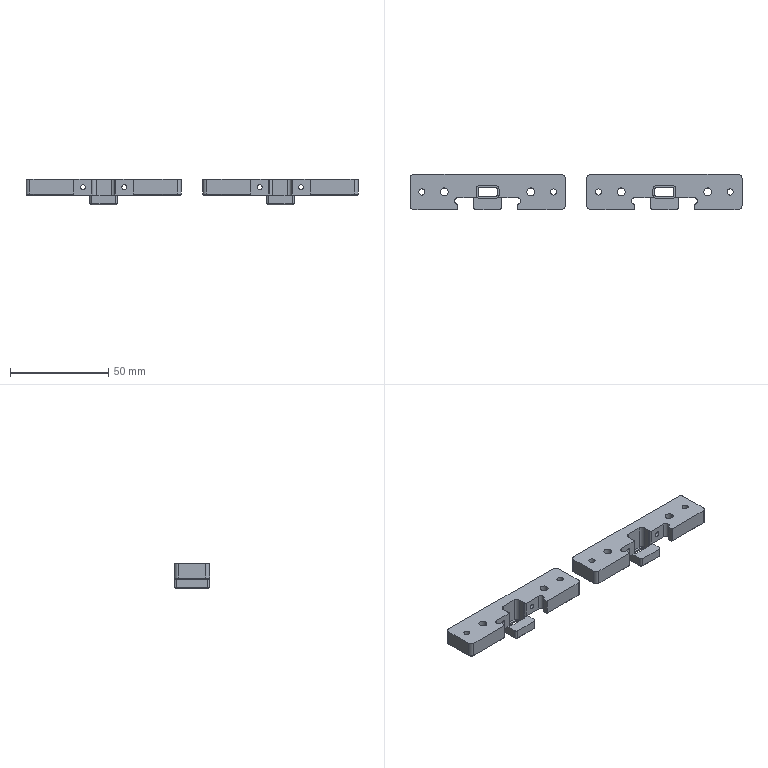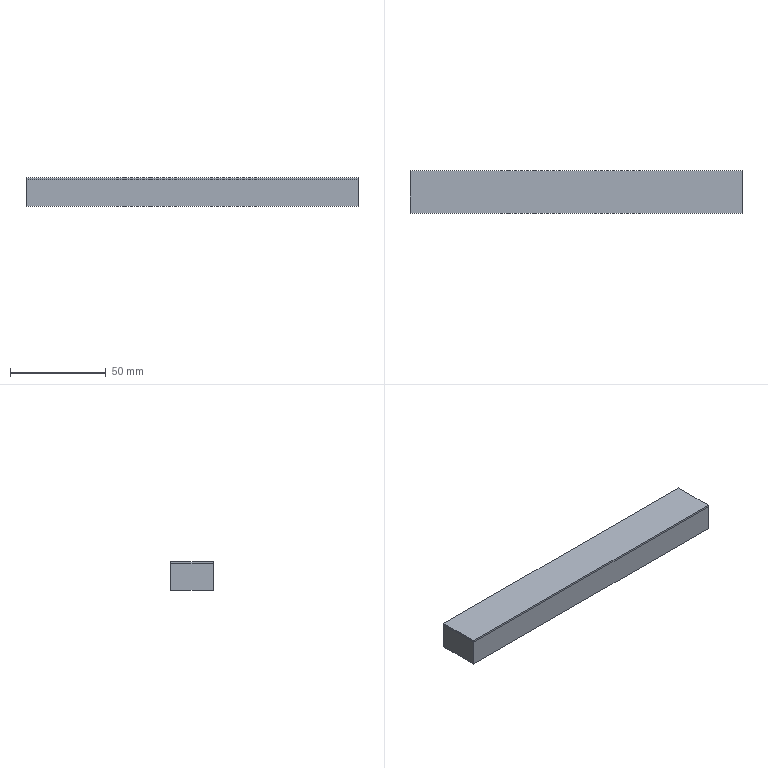CAM job | NX | 3-axis milling, drilling | part box 169 x 18 x 12.9 mm | stock box 173 x 22 x 14.9 mm
Tools:
number,name,description,diameter,corner_radius,flute_length,length,flutes
1,D63,Milling Tool-5 Parameters,63.0,0.0,50.0,75.0,2
2,D4A45,Milling Tool-5 Parameters,4.0,0.0,2.0,2.0,2
13,3.1ZT,Drilling Tool,3.1,0.0,35.0,50.0,2
14,4.1ZT,Drilling Tool,4.1,0.0,35.0,50.0,2
6,D6,Milling Tool-5 Parameters,6.0,0.0,50.0,75.0,2
4,D4,Milling Tool-5 Parameters,4.0,0.0,50.0,75.0,2
3,D3,Milling Tool-5 Parameters,3.0,0.0,50.0,75.0,2
12,D2,Milling Tool-5 Parameters,2.0,0.0,50.0,75.0,2
Operations:
program,operation,operation_type,tool,method,geometry_group,spindle_rpm,surface_speed,feed_per_tooth,feed_cut,feed_plunge,cut_length_mm,path_length_mm,cut_time_min,machine_time_min
1虎钳,FLOOR_WALL,VolumeBased25DMillingOperation,D63,METHOD,A,6500.0,1286.0,0.0962,1250.0,100.0,248.0,302.0,0.1984,0.2038
1虎钳,DRILLING_COPY,Operation,D4A45,METHOD,A,5000.0,62.0,0.025,250.0,0.0,28.8,297.539,0.1152,0.1421
1虎钳,DRILLING_COPY_COPY_COPY_COPY_COPY_COPY_1,Operation,3.1ZT,METHOD,A,1910.0,21.0,0.0471,180.0,0.0,47.725,321.78,0.2651,0.2925
1虎钳,DRILLING_COPY_COPY_COPY_COPY_COPY_COPY_1_COPY,Operation,4.1ZT,METHOD,A,1910.0,21.0,0.0471,180.0,0.0,52.927,309.156,0.294,0.3197
1虎钳,ZLEVEL_PROFILE_COPY_COPY_1_COPY,ZLevelMilling,D6,METHOD,A,9500.0,179.0,0.1158,2200.0,1000.0,7428.489,7715.293,3.418,3.447
1虎钳,ZLEVEL_PROFILE_COPY_COPY_1_COPY_COPY_COPY_1_COPY,ZLevelMilling,D6,METHOD,A,9500.0,179.0,0.1158,2200.0,1000.0,1035.18,1277.296,0.498,0.5223
1虎钳,ZLEVEL_PROFILE_COPY_COPY_1_COPY_COPY_COPY_1,ZLevelMilling,D6,METHOD,A,9500.0,179.0,0.1158,2200.0,1000.0,1574.227,1816.224,0.744,0.7682
1虎钳,ZLEVEL_PROFILE_COPY_COPY_1_COPY_COPY,ZLevelMilling,D6,METHOD,A,9500.0,179.0,0.1158,2200.0,1000.0,319.802,561.779,0.1864,0.2106
1虎钳,CAVITY_MILL_COPY_COPY,CavityMilling,D4,METHOD,A,9500.0,119.0,0.1053,2000.0,1000.0,1753.784,4067.341,1.101,1.332
1虎钳,ZLEVEL_PROFILE_COPY_COPY_1_COPY_COPY_COPY,ZLevelMilling,D4,METHOD,A,9500.0,179.0,0.1158,2200.0,1000.0,146.243,395.295,0.105,0.1299
1虎钳,CAVITY_MILL_COPY_COPY_COPY,CavityMilling,D3,METHOD,A,9500.0,89.0,0.0632,1200.0,1000.0,1401.506,3153.601,1.217,1.393
1虎钳,CAVITY_MILL_COPY_COPY_COPY_COPY,CavityMilling,D2,METHOD,A,9500.0,89.0,0.0632,1200.0,1000.0,107.206,923.977,0.0943,0.176
1虎钳,ZLEVEL_PROFILE_COPY_COPY_COPY_COPY,ZLevelMilling,D4,MILL_FINISH,A,9500.0,119.0,0.0632,1200.0,1000.0,459.893,694.983,0.384,0.4075
1虎钳,ZLEVEL_PROFILE_COPY_COPY_COPY_COPY_COPY,ZLevelMilling,D4,MILL_FINISH,A,9500.0,119.0,0.0632,1200.0,1000.0,50.928,303.784,0.0432,0.0684
1虎钳,ZLEVEL_PROFILE_1_COPY_1_COPY_COPY,ZLevelMilling,D4A45,METHOD,A,9500.0,179.0,0.0526,1000.0,100.0,528.005,1607.183,0.528,0.6359
2,FLOOR_WALL_COPY,VolumeBased25DMillingOperation,D63,METHOD,B,6500.0,1286.0,0.0962,1250.0,100.0,496.0,844,0.3968,0.4316
2,CAVITY_MILL_COPY_COPY_COPY_1,CavityMilling,D6,METHOD,B,9500.0,179.0,0.1053,2000.0,1000.0,10825.153,11453.098,5.433,5.495
2,ZLEVEL_PROFILE_COPY_COPY_COPY_COPY_COPY_COPY,ZLevelMilling,D6,MILL_FINISH,B,9500.0,119.0,0.0632,1200.0,1000.0,172.053,376.329,0.1442,0.1646
2,FLOOR_WALL_1,VolumeBased25DMillingOperation,D6,METHOD,B,9500.0,119.0,0.0526,1000.0,100.0,1220.866,1942.476,1.221,1.293
2,HOLE_MILLING,CylinderMilling,D4,METHOD,B,9500.0,179.0,0.0789,1500.0,100.0,321.015,771.215,0.214,0.259
2,ZLEVEL_PROFILE_1_COPY_1_COPY_COPY_COPY,ZLevelMilling,D4A45,METHOD,B,9500.0,179.0,0.0526,1000.0,100.0,190.621,605.531,0.1906,0.2321
2,ZLEVEL_PROFILE_1_COPY_1_COPY_COPY_COPY_COPY,ZLevelMilling,D4A45,METHOD,B,9500.0,179.0,0.0526,1000.0,100.0,476.39,1846.56,0.4764,0.6134